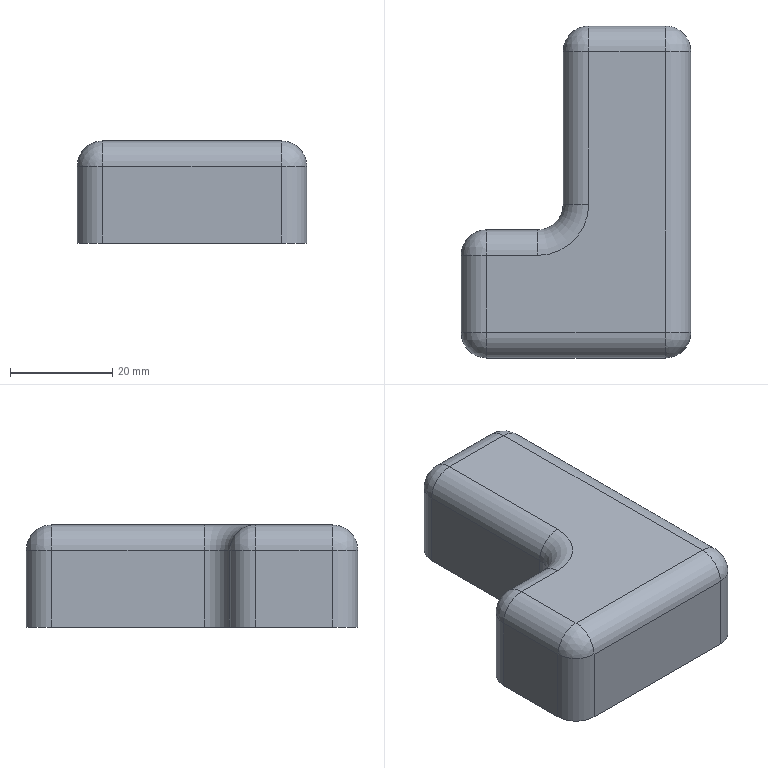Part | SolidWorks | features BaseBody 1 | 1 solid | 26 faces | box 45 x 65 x 20 mm | volume 41025 mm3 | cylinder 12 | plane 8 | sphere 5 | torus 1 | commonest cylinder face diameters 10 x12
STEP:
#1=CARTESIAN_POINT('',(40.,0.,15.));
#2=VERTEX_POINT('',#1);
#3=CARTESIAN_POINT('',(5.,0.,15.));
#4=VERTEX_POINT('',#3);
#5=CARTESIAN_POINT('',(45.,0.,15.));
#6=DIRECTION('',(-1.,0.,0.));
#7=VECTOR('',#6,1000.);
#8=LINE('',#5,#7);
#9=EDGE_CURVE('',#2,#4,#8,.T.);
#10=ORIENTED_EDGE('',*,*,#9,.T.);
#11=CARTESIAN_POINT('',(5.,0.,0.));
#12=VERTEX_POINT('',#11);
#13=CARTESIAN_POINT('',(5.,0.,20.));
#14=DIRECTION('',(0.,0.,-1.));
#15=VECTOR('',#14,1000.);
#16=LINE('',#13,#15);
#17=EDGE_CURVE('',#4,#12,#16,.T.);
#18=ORIENTED_EDGE('',*,*,#17,.T.);
#19=CARTESIAN_POINT('',(40.,0.,0.));
#20=VERTEX_POINT('',#19);
#21=CARTESIAN_POINT('',(45.,0.,0.));
#22=DIRECTION('',(1.,0.,0.));
#23=VECTOR('',#22,1000.);
#24=LINE('',#21,#23);
#25=EDGE_CURVE('',#12,#20,#24,.T.);
#26=ORIENTED_EDGE('',*,*,#25,.T.);
#27=CARTESIAN_POINT('',(40.,0.,20.));
#28=DIRECTION('',(0.,0.,1.));
#29=VECTOR('',#28,1000.);
#30=LINE('',#27,#29);
#31=EDGE_CURVE('',#20,#2,#30,.T.);
#32=ORIENTED_EDGE('',*,*,#31,.T.);
#33=EDGE_LOOP('',(#10,#18,#26,#32));
#34=FACE_OUTER_BOUND('',#33,.T.);
#35=CARTESIAN_POINT('',(45.,0.,20.));
#36=DIRECTION('',(0.,1.,0.));
#37=DIRECTION('',(-1.,0.,0.));
#38=AXIS2_PLACEMENT_3D('',#35,#36,#37);
#39=PLANE('',#38);
#40=ADVANCED_FACE('',(#34),#39,.F.);
#41=CARTESIAN_POINT('',(45.,60.,15.));
#42=VERTEX_POINT('',#41);
#43=CARTESIAN_POINT('',(45.,5.,15.));
#44=VERTEX_POINT('',#43);
#45=CARTESIAN_POINT('',(45.,65.,15.));
#46=DIRECTION('',(0.,-1.,0.));
#47=VECTOR('',#46,1000.);
#48=LINE('',#45,#47);
#49=EDGE_CURVE('',#42,#44,#48,.T.);
#50=ORIENTED_EDGE('',*,*,#49,.T.);
#51=CARTESIAN_POINT('',(45.,5.,0.));
#52=VERTEX_POINT('',#51);
#53=CARTESIAN_POINT('',(45.,5.,20.));
#54=DIRECTION('',(0.,0.,-1.));
#55=VECTOR('',#54,1000.);
#56=LINE('',#53,#55);
#57=EDGE_CURVE('',#44,#52,#56,.T.);
#58=ORIENTED_EDGE('',*,*,#57,.T.);
#59=CARTESIAN_POINT('',(45.,60.,0.));
#60=VERTEX_POINT('',#59);
#61=CARTESIAN_POINT('',(45.,65.,0.));
#62=DIRECTION('',(0.,1.,0.));
#63=VECTOR('',#62,1000.);
#64=LINE('',#61,#63);
#65=EDGE_CURVE('',#52,#60,#64,.T.);
#66=ORIENTED_EDGE('',*,*,#65,.T.);
#67=CARTESIAN_POINT('',(45.,60.,20.));
#68=DIRECTION('',(0.,0.,1.));
#69=VECTOR('',#68,1000.);
#70=LINE('',#67,#69);
#71=EDGE_CURVE('',#60,#42,#70,.T.);
#72=ORIENTED_EDGE('',*,*,#71,.T.);
#73=EDGE_LOOP('',(#50,#58,#66,#72));
#74=FACE_OUTER_BOUND('',#73,.T.);
#75=CARTESIAN_POINT('',(45.,65.,20.));
#76=DIRECTION('',(-1.,0.,0.));
#77=DIRECTION('',(0.,-1.,0.));
#78=AXIS2_PLACEMENT_3D('',#75,#76,#77);
#79=PLANE('',#78);
#80=ADVANCED_FACE('',(#74),#79,.F.);
#81=CARTESIAN_POINT('',(25.,65.,15.));
#82=VERTEX_POINT('',#81);
#83=CARTESIAN_POINT('',(40.,65.,15.));
#84=VERTEX_POINT('',#83);
#85=CARTESIAN_POINT('',(20.,65.,15.));
#86=DIRECTION('',(1.,0.,0.));
#87=VECTOR('',#86,1000.);
#88=LINE('',#85,#87);
#89=EDGE_CURVE('',#82,#84,#88,.T.);
#90=ORIENTED_EDGE('',*,*,#89,.T.);
#91=CARTESIAN_POINT('',(40.,65.,0.));
#92=VERTEX_POINT('',#91);
#93=CARTESIAN_POINT('',(40.,65.,20.));
#94=DIRECTION('',(0.,0.,-1.));
#95=VECTOR('',#94,1000.);
#96=LINE('',#93,#95);
#97=EDGE_CURVE('',#84,#92,#96,.T.);
#98=ORIENTED_EDGE('',*,*,#97,.T.);
#99=CARTESIAN_POINT('',(25.,65.,0.));
#100=VERTEX_POINT('',#99);
#101=CARTESIAN_POINT('',(20.,65.,0.));
#102=DIRECTION('',(-1.,0.,0.));
#103=VECTOR('',#102,1000.);
#104=LINE('',#101,#103);
#105=EDGE_CURVE('',#92,#100,#104,.T.);
#106=ORIENTED_EDGE('',*,*,#105,.T.);
#107=CARTESIAN_POINT('',(25.,65.,20.));
#108=DIRECTION('',(0.,0.,1.));
#109=VECTOR('',#108,1000.);
#110=LINE('',#107,#109);
#111=EDGE_CURVE('',#100,#82,#110,.T.);
#112=ORIENTED_EDGE('',*,*,#111,.T.);
#113=EDGE_LOOP('',(#90,#98,#106,#112));
#114=FACE_OUTER_BOUND('',#113,.T.);
#115=CARTESIAN_POINT('',(20.,65.,20.));
#116=DIRECTION('',(0.,-1.,0.));
#117=DIRECTION('',(0.,0.,-1.));
#118=AXIS2_PLACEMENT_3D('',#115,#116,#117);
#119=PLANE('',#118);
#120=ADVANCED_FACE('',(#114),#119,.F.);
#121=CARTESIAN_POINT('',(20.,30.07,15.));
#122=VERTEX_POINT('',#121);
#123=CARTESIAN_POINT('',(20.,60.,15.));
#124=VERTEX_POINT('',#123);
#125=CARTESIAN_POINT('',(20.,25.07,15.));
#126=DIRECTION('',(0.,1.,0.));
#127=VECTOR('',#126,1000.);
#128=LINE('',#125,#127);
#129=EDGE_CURVE('',#122,#124,#128,.T.);
#130=ORIENTED_EDGE('',*,*,#129,.T.);
#131=CARTESIAN_POINT('',(20.,60.,0.));
#132=VERTEX_POINT('',#131);
#133=CARTESIAN_POINT('',(20.,60.,20.));
#134=DIRECTION('',(0.,0.,-1.));
#135=VECTOR('',#134,1000.);
#136=LINE('',#133,#135);
#137=EDGE_CURVE('',#124,#132,#136,.T.);
#138=ORIENTED_EDGE('',*,*,#137,.T.);
#139=CARTESIAN_POINT('',(20.,30.07,0.));
#140=VERTEX_POINT('',#139);
#141=CARTESIAN_POINT('',(20.,25.07,0.));
#142=DIRECTION('',(0.,-1.,0.));
#143=VECTOR('',#142,1000.);
#144=LINE('',#141,#143);
#145=EDGE_CURVE('',#132,#140,#144,.T.);
#146=ORIENTED_EDGE('',*,*,#145,.T.);
#147=CARTESIAN_POINT('',(20.,30.07,20.));
#148=DIRECTION('',(0.,0.,1.));
#149=VECTOR('',#148,1000.);
#150=LINE('',#147,#149);
#151=EDGE_CURVE('',#140,#122,#150,.T.);
#152=ORIENTED_EDGE('',*,*,#151,.T.);
#153=EDGE_LOOP('',(#130,#138,#146,#152));
#154=FACE_OUTER_BOUND('',#153,.T.);
#155=CARTESIAN_POINT('',(20.,25.07,20.));
#156=DIRECTION('',(1.,0.,0.));
#157=DIRECTION('',(0.,0.,-1.));
#158=AXIS2_PLACEMENT_3D('',#155,#156,#157);
#159=PLANE('',#158);
#160=ADVANCED_FACE('',(#154),#159,.F.);
#161=CARTESIAN_POINT('',(5.,25.07,15.));
#162=VERTEX_POINT('',#161);
#163=CARTESIAN_POINT('',(15.,25.07,15.));
#164=VERTEX_POINT('',#163);
#165=CARTESIAN_POINT('',(0.,25.07,15.));
#166=DIRECTION('',(1.,0.,0.));
#167=VECTOR('',#166,1000.);
#168=LINE('',#165,#167);
#169=EDGE_CURVE('',#162,#164,#168,.T.);
#170=ORIENTED_EDGE('',*,*,#169,.T.);
#171=CARTESIAN_POINT('',(15.,25.07,0.));
#172=VERTEX_POINT('',#171);
#173=CARTESIAN_POINT('',(15.,25.07,0.));
#174=DIRECTION('',(0.,0.,-1.));
#175=VECTOR('',#174,1000.);
#176=LINE('',#173,#175);
#177=EDGE_CURVE('',#164,#172,#176,.T.);
#178=ORIENTED_EDGE('',*,*,#177,.T.);
#179=CARTESIAN_POINT('',(5.,25.07,0.));
#180=VERTEX_POINT('',#179);
#181=CARTESIAN_POINT('',(0.,25.07,0.));
#182=DIRECTION('',(-1.,0.,0.));
#183=VECTOR('',#182,1000.);
#184=LINE('',#181,#183);
#185=EDGE_CURVE('',#172,#180,#184,.T.);
#186=ORIENTED_EDGE('',*,*,#185,.T.);
#187=CARTESIAN_POINT('',(5.,25.07,20.));
#188=DIRECTION('',(0.,0.,1.));
#189=VECTOR('',#188,1000.);
#190=LINE('',#187,#189);
#191=EDGE_CURVE('',#180,#162,#190,.T.);
#192=ORIENTED_EDGE('',*,*,#191,.T.);
#193=EDGE_LOOP('',(#170,#178,#186,#192));
#194=FACE_OUTER_BOUND('',#193,.T.);
#195=CARTESIAN_POINT('',(0.,25.07,20.));
#196=DIRECTION('',(0.,-1.,0.));
#197=DIRECTION('',(0.,0.,-1.));
#198=AXIS2_PLACEMENT_3D('',#195,#196,#197);
#199=PLANE('',#198);
#200=ADVANCED_FACE('',(#194),#199,.F.);
#201=CARTESIAN_POINT('',(0.,20.07,0.));
#202=VERTEX_POINT('',#201);
#203=CARTESIAN_POINT('',(0.,5.,0.));
#204=VERTEX_POINT('',#203);
#205=CARTESIAN_POINT('',(0.,0.,0.));
#206=DIRECTION('',(0.,-1.,0.));
#207=VECTOR('',#206,1000.);
#208=LINE('',#205,#207);
#209=EDGE_CURVE('',#202,#204,#208,.T.);
#210=ORIENTED_EDGE('',*,*,#209,.T.);
#211=CARTESIAN_POINT('',(0.,5.,15.));
#212=VERTEX_POINT('',#211);
#213=CARTESIAN_POINT('',(0.,5.,20.));
#214=DIRECTION('',(0.,0.,1.));
#215=VECTOR('',#214,1000.);
#216=LINE('',#213,#215);
#217=EDGE_CURVE('',#204,#212,#216,.T.);
#218=ORIENTED_EDGE('',*,*,#217,.T.);
#219=CARTESIAN_POINT('',(0.,20.07,15.));
#220=VERTEX_POINT('',#219);
#221=CARTESIAN_POINT('',(0.,0.,15.));
#222=DIRECTION('',(0.,1.,0.));
#223=VECTOR('',#222,1000.);
#224=LINE('',#221,#223);
#225=EDGE_CURVE('',#212,#220,#224,.T.);
#226=ORIENTED_EDGE('',*,*,#225,.T.);
#227=CARTESIAN_POINT('',(0.,20.07,20.));
#228=DIRECTION('',(0.,0.,-1.));
#229=VECTOR('',#228,1000.);
#230=LINE('',#227,#229);
#231=EDGE_CURVE('',#220,#202,#230,.T.);
#232=ORIENTED_EDGE('',*,*,#231,.T.);
#233=EDGE_LOOP('',(#210,#218,#226,#232));
#234=FACE_OUTER_BOUND('',#233,.T.);
#235=CARTESIAN_POINT('',(0.,0.,20.));
#236=DIRECTION('',(1.,0.,0.));
#237=DIRECTION('',(0.,0.,-1.));
#238=AXIS2_PLACEMENT_3D('',#235,#236,#237);
#239=PLANE('',#238);
#240=ADVANCED_FACE('',(#234),#239,.F.);
#241=CARTESIAN_POINT('',(40.,60.,20.));
#242=VERTEX_POINT('',#241);
#243=CARTESIAN_POINT('',(25.,60.,20.));
#244=VERTEX_POINT('',#243);
#245=CARTESIAN_POINT('',(0.,60.,20.));
#246=DIRECTION('',(-1.,0.,0.));
#247=VECTOR('',#246,1000.);
#248=LINE('',#245,#247);
#249=EDGE_CURVE('',#242,#244,#248,.T.);
#250=ORIENTED_EDGE('',*,*,#249,.T.);
#251=CARTESIAN_POINT('',(25.,30.07,20.));
#252=VERTEX_POINT('',#251);
#253=CARTESIAN_POINT('',(25.,0.,20.));
#254=DIRECTION('',(0.,-1.,0.));
#255=VECTOR('',#254,1000.);
#256=LINE('',#253,#255);
#257=EDGE_CURVE('',#244,#252,#256,.T.);
#258=ORIENTED_EDGE('',*,*,#257,.T.);
#259=CARTESIAN_POINT('',(15.,20.07,20.));
#260=VERTEX_POINT('',#259);
#261=CARTESIAN_POINT('',(15.,30.07,20.));
#262=DIRECTION('',(0.,0.,1.));
#263=DIRECTION('',(-1.,0.,0.));
#264=AXIS2_PLACEMENT_3D('',#261,#262,#263);
#265=CIRCLE('',#264,10.);
#266=EDGE_CURVE('',#260,#252,#265,.T.);
#267=ORIENTED_EDGE('',*,*,#266,.F.);
#268=CARTESIAN_POINT('',(5.,20.07,20.));
#269=VERTEX_POINT('',#268);
#270=CARTESIAN_POINT('',(0.,20.07,20.));
#271=DIRECTION('',(-1.,0.,0.));
#272=VECTOR('',#271,1000.);
#273=LINE('',#270,#272);
#274=EDGE_CURVE('',#260,#269,#273,.T.);
#275=ORIENTED_EDGE('',*,*,#274,.T.);
#276=CARTESIAN_POINT('',(5.,5.,20.));
#277=VERTEX_POINT('',#276);
#278=CARTESIAN_POINT('',(5.,0.,20.));
#279=DIRECTION('',(0.,-1.,0.));
#280=VECTOR('',#279,1000.);
#281=LINE('',#278,#280);
#282=EDGE_CURVE('',#269,#277,#281,.T.);
#283=ORIENTED_EDGE('',*,*,#282,.T.);
#284=CARTESIAN_POINT('',(40.,5.,20.));
#285=VERTEX_POINT('',#284);
#286=CARTESIAN_POINT('',(0.,5.,20.));
#287=DIRECTION('',(1.,0.,0.));
#288=VECTOR('',#287,1000.);
#289=LINE('',#286,#288);
#290=EDGE_CURVE('',#277,#285,#289,.T.);
#291=ORIENTED_EDGE('',*,*,#290,.T.);
#292=CARTESIAN_POINT('',(40.,0.,20.));
#293=DIRECTION('',(0.,1.,0.));
#294=VECTOR('',#293,1000.);
#295=LINE('',#292,#294);
#296=EDGE_CURVE('',#285,#242,#295,.T.);
#297=ORIENTED_EDGE('',*,*,#296,.T.);
#298=EDGE_LOOP('',(#250,#258,#267,#275,#283,#291,#297));
#299=FACE_OUTER_BOUND('',#298,.T.);
#300=CARTESIAN_POINT('',(0.,0.,20.));
#301=DIRECTION('',(0.,0.,-1.));
#302=DIRECTION('',(-1.,0.,0.));
#303=AXIS2_PLACEMENT_3D('',#300,#301,#302);
#304=PLANE('',#303);
#305=ADVANCED_FACE('',(#299),#304,.F.);
#306=ORIENTED_EDGE('',*,*,#25,.F.);
#307=CARTESIAN_POINT('',(5.,5.,0.));
#308=DIRECTION('',(0.,0.,-1.));
#309=DIRECTION('',(-1.,0.,0.));
#310=AXIS2_PLACEMENT_3D('',#307,#308,#309);
#311=CIRCLE('',#310,5.);
#312=EDGE_CURVE('',#12,#204,#311,.T.);
#313=ORIENTED_EDGE('',*,*,#312,.T.);
#314=ORIENTED_EDGE('',*,*,#209,.F.);
#315=CARTESIAN_POINT('',(5.,20.07,0.));
#316=DIRECTION('',(0.,0.,-1.));
#317=DIRECTION('',(-1.,0.,0.));
#318=AXIS2_PLACEMENT_3D('',#315,#316,#317);
#319=CIRCLE('',#318,5.);
#320=EDGE_CURVE('',#202,#180,#319,.T.);
#321=ORIENTED_EDGE('',*,*,#320,.T.);
#322=ORIENTED_EDGE('',*,*,#185,.F.);
#323=CARTESIAN_POINT('',(15.,30.07,0.));
#324=DIRECTION('',(0.,0.,1.));
#325=DIRECTION('',(-1.,0.,0.));
#326=AXIS2_PLACEMENT_3D('',#323,#324,#325);
#327=CIRCLE('',#326,5.);
#328=EDGE_CURVE('',#172,#140,#327,.T.);
#329=ORIENTED_EDGE('',*,*,#328,.T.);
#330=ORIENTED_EDGE('',*,*,#145,.F.);
#331=CARTESIAN_POINT('',(25.,60.,0.));
#332=DIRECTION('',(0.,0.,-1.));
#333=DIRECTION('',(-1.,0.,0.));
#334=AXIS2_PLACEMENT_3D('',#331,#332,#333);
#335=CIRCLE('',#334,5.);
#336=EDGE_CURVE('',#132,#100,#335,.T.);
#337=ORIENTED_EDGE('',*,*,#336,.T.);
#338=ORIENTED_EDGE('',*,*,#105,.F.);
#339=CARTESIAN_POINT('',(40.,60.,0.));
#340=DIRECTION('',(0.,0.,-1.));
#341=DIRECTION('',(-1.,0.,0.));
#342=AXIS2_PLACEMENT_3D('',#339,#340,#341);
#343=CIRCLE('',#342,5.);
#344=EDGE_CURVE('',#92,#60,#343,.T.);
#345=ORIENTED_EDGE('',*,*,#344,.T.);
#346=ORIENTED_EDGE('',*,*,#65,.F.);
#347=CARTESIAN_POINT('',(40.,5.,0.));
#348=DIRECTION('',(0.,0.,-1.));
#349=DIRECTION('',(-1.,0.,0.));
#350=AXIS2_PLACEMENT_3D('',#347,#348,#349);
#351=CIRCLE('',#350,5.);
#352=EDGE_CURVE('',#52,#20,#351,.T.);
#353=ORIENTED_EDGE('',*,*,#352,.T.);
#354=EDGE_LOOP('',(#306,#313,#314,#321,#322,#329,#330,#337,#338,#345,#346,#353));
#355=FACE_OUTER_BOUND('',#354,.T.);
#356=CARTESIAN_POINT('',(0.,0.,0.));
#357=DIRECTION('',(0.,0.,-1.));
#358=DIRECTION('',(-1.,0.,0.));
#359=AXIS2_PLACEMENT_3D('',#356,#357,#358);
#360=PLANE('',#359);
#361=ADVANCED_FACE('',(#355),#360,.T.);
#362=ORIENTED_EDGE('',*,*,#352,.F.);
#363=ORIENTED_EDGE('',*,*,#57,.F.);
#364=CARTESIAN_POINT('',(40.,5.,15.));
#365=DIRECTION('',(0.,0.,1.));
#366=DIRECTION('',(1.,0.,0.));
#367=AXIS2_PLACEMENT_3D('',#364,#365,#366);
#368=CIRCLE('',#367,5.);
#369=EDGE_CURVE('',#2,#44,#368,.T.);
#370=ORIENTED_EDGE('',*,*,#369,.F.);
#371=ORIENTED_EDGE('',*,*,#31,.F.);
#372=EDGE_LOOP('',(#362,#363,#370,#371));
#373=FACE_OUTER_BOUND('',#372,.T.);
#374=CARTESIAN_POINT('',(40.,5.,20.));
#375=DIRECTION('',(0.,0.,-1.));
#376=DIRECTION('',(-1.,0.,0.));
#377=AXIS2_PLACEMENT_3D('',#374,#375,#376);
#378=CYLINDRICAL_SURFACE('',#377,5.);
#379=ADVANCED_FACE('',(#373),#378,.T.);
#380=CARTESIAN_POINT('',(5.,5.,15.));
#381=DIRECTION('',(-1.,0.,0.));
#382=DIRECTION('',(0.,0.,1.));
#383=AXIS2_PLACEMENT_3D('',#380,#381,#382);
#384=CIRCLE('',#383,5.);
#385=EDGE_CURVE('',#4,#277,#384,.T.);
#386=ORIENTED_EDGE('',*,*,#385,.F.);
#387=ORIENTED_EDGE('',*,*,#9,.F.);
#388=CARTESIAN_POINT('',(40.,5.,15.));
#389=DIRECTION('',(1.,0.,0.));
#390=DIRECTION('',(0.,0.,-1.));
#391=AXIS2_PLACEMENT_3D('',#388,#389,#390);
#392=CIRCLE('',#391,5.);
#393=EDGE_CURVE('',#285,#2,#392,.T.);
#394=ORIENTED_EDGE('',*,*,#393,.F.);
#395=ORIENTED_EDGE('',*,*,#290,.F.);
#396=EDGE_LOOP('',(#386,#387,#394,#395));
#397=FACE_OUTER_BOUND('',#396,.T.);
#398=CARTESIAN_POINT('',(0.,5.,15.));
#399=DIRECTION('',(1.,0.,0.));
#400=DIRECTION('',(0.,1.,0.));
#401=AXIS2_PLACEMENT_3D('',#398,#399,#400);
#402=CYLINDRICAL_SURFACE('',#401,5.);
#403=ADVANCED_FACE('',(#397),#402,.T.);
#404=ORIENTED_EDGE('',*,*,#312,.F.);
#405=ORIENTED_EDGE('',*,*,#17,.F.);
#406=CARTESIAN_POINT('',(5.,5.,15.));
#407=DIRECTION('',(0.,0.,1.));
#408=DIRECTION('',(1.,0.,0.));
#409=AXIS2_PLACEMENT_3D('',#406,#407,#408);
#410=CIRCLE('',#409,5.);
#411=EDGE_CURVE('',#212,#4,#410,.T.);
#412=ORIENTED_EDGE('',*,*,#411,.F.);
#413=ORIENTED_EDGE('',*,*,#217,.F.);
#414=EDGE_LOOP('',(#404,#405,#412,#413));
#415=FACE_OUTER_BOUND('',#414,.T.);
#416=CARTESIAN_POINT('',(5.,5.,20.));
#417=DIRECTION('',(0.,0.,-1.));
#418=DIRECTION('',(-1.,0.,0.));
#419=AXIS2_PLACEMENT_3D('',#416,#417,#418);
#420=CYLINDRICAL_SURFACE('',#419,5.);
#421=ADVANCED_FACE('',(#415),#420,.T.);
#422=ORIENTED_EDGE('',*,*,#393,.T.);
#423=ORIENTED_EDGE('',*,*,#369,.T.);
#424=CARTESIAN_POINT('',(40.,5.,15.));
#425=DIRECTION('',(0.,1.,0.));
#426=DIRECTION('',(0.,0.,-1.));
#427=AXIS2_PLACEMENT_3D('',#424,#425,#426);
#428=CIRCLE('',#427,5.);
#429=EDGE_CURVE('',#285,#44,#428,.T.);
#430=ORIENTED_EDGE('',*,*,#429,.F.);
#431=EDGE_LOOP('',(#422,#423,#430));
#432=FACE_OUTER_BOUND('',#431,.T.);
#433=CARTESIAN_POINT('',(40.,5.,15.));
#434=DIRECTION('',(0.,1.,0.));
#435=DIRECTION('',(1.,0.,0.));
#436=AXIS2_PLACEMENT_3D('',#433,#434,#435);
#437=SPHERICAL_SURFACE('',#436,5.);
#438=ADVANCED_FACE('',(#432),#437,.T.);
#439=ORIENTED_EDGE('',*,*,#411,.T.);
#440=ORIENTED_EDGE('',*,*,#385,.T.);
#441=CARTESIAN_POINT('',(5.,5.,15.));
#442=DIRECTION('',(0.,1.,0.));
#443=DIRECTION('',(0.,0.,-1.));
#444=AXIS2_PLACEMENT_3D('',#441,#442,#443);
#445=CIRCLE('',#444,5.);
#446=EDGE_CURVE('',#212,#277,#445,.T.);
#447=ORIENTED_EDGE('',*,*,#446,.F.);
#448=EDGE_LOOP('',(#439,#440,#447));
#449=FACE_OUTER_BOUND('',#448,.T.);
#450=CARTESIAN_POINT('',(5.,5.,15.));
#451=DIRECTION('',(0.,1.,0.));
#452=DIRECTION('',(1.,0.,0.));
#453=AXIS2_PLACEMENT_3D('',#450,#451,#452);
#454=SPHERICAL_SURFACE('',#453,5.);
#455=ADVANCED_FACE('',(#449),#454,.T.);
#456=ORIENTED_EDGE('',*,*,#344,.F.);
#457=ORIENTED_EDGE('',*,*,#97,.F.);
#458=CARTESIAN_POINT('',(40.,60.,15.));
#459=DIRECTION('',(0.,0.,1.));
#460=DIRECTION('',(1.,0.,0.));
#461=AXIS2_PLACEMENT_3D('',#458,#459,#460);
#462=CIRCLE('',#461,5.);
#463=EDGE_CURVE('',#42,#84,#462,.T.);
#464=ORIENTED_EDGE('',*,*,#463,.F.);
#465=ORIENTED_EDGE('',*,*,#71,.F.);
#466=EDGE_LOOP('',(#456,#457,#464,#465));
#467=FACE_OUTER_BOUND('',#466,.T.);
#468=CARTESIAN_POINT('',(40.,60.,20.));
#469=DIRECTION('',(0.,0.,-1.));
#470=DIRECTION('',(-1.,0.,0.));
#471=AXIS2_PLACEMENT_3D('',#468,#469,#470);
#472=CYLINDRICAL_SURFACE('',#471,5.);
#473=ADVANCED_FACE('',(#467),#472,.T.);
#474=ORIENTED_EDGE('',*,*,#429,.T.);
#475=ORIENTED_EDGE('',*,*,#49,.F.);
#476=CARTESIAN_POINT('',(40.,60.,15.));
#477=DIRECTION('',(0.,1.,0.));
#478=DIRECTION('',(0.,0.,1.));
#479=AXIS2_PLACEMENT_3D('',#476,#477,#478);
#480=CIRCLE('',#479,5.);
#481=EDGE_CURVE('',#242,#42,#480,.T.);
#482=ORIENTED_EDGE('',*,*,#481,.F.);
#483=ORIENTED_EDGE('',*,*,#296,.F.);
#484=EDGE_LOOP('',(#474,#475,#482,#483));
#485=FACE_OUTER_BOUND('',#484,.T.);
#486=CARTESIAN_POINT('',(40.,0.,15.));
#487=DIRECTION('',(0.,1.,0.));
#488=DIRECTION('',(-1.,0.,0.));
#489=AXIS2_PLACEMENT_3D('',#486,#487,#488);
#490=CYLINDRICAL_SURFACE('',#489,5.);
#491=ADVANCED_FACE('',(#485),#490,.T.);
#492=ORIENTED_EDGE('',*,*,#446,.T.);
#493=ORIENTED_EDGE('',*,*,#282,.F.);
#494=CARTESIAN_POINT('',(5.,20.07,15.));
#495=DIRECTION('',(0.,1.,0.));
#496=DIRECTION('',(0.,0.,1.));
#497=AXIS2_PLACEMENT_3D('',#494,#495,#496);
#498=CIRCLE('',#497,5.);
#499=EDGE_CURVE('',#220,#269,#498,.T.);
#500=ORIENTED_EDGE('',*,*,#499,.F.);
#501=ORIENTED_EDGE('',*,*,#225,.F.);
#502=EDGE_LOOP('',(#492,#493,#500,#501));
#503=FACE_OUTER_BOUND('',#502,.T.);
#504=CARTESIAN_POINT('',(5.,0.,15.));
#505=DIRECTION('',(0.,-1.,0.));
#506=DIRECTION('',(0.,0.,-1.));
#507=AXIS2_PLACEMENT_3D('',#504,#505,#506);
#508=CYLINDRICAL_SURFACE('',#507,5.);
#509=ADVANCED_FACE('',(#503),#508,.T.);
#510=ORIENTED_EDGE('',*,*,#320,.F.);
#511=ORIENTED_EDGE('',*,*,#231,.F.);
#512=CARTESIAN_POINT('',(5.,20.07,15.));
#513=DIRECTION('',(0.,0.,1.));
#514=DIRECTION('',(1.,0.,0.));
#515=AXIS2_PLACEMENT_3D('',#512,#513,#514);
#516=CIRCLE('',#515,5.);
#517=EDGE_CURVE('',#162,#220,#516,.T.);
#518=ORIENTED_EDGE('',*,*,#517,.F.);
#519=ORIENTED_EDGE('',*,*,#191,.F.);
#520=EDGE_LOOP('',(#510,#511,#518,#519));
#521=FACE_OUTER_BOUND('',#520,.T.);
#522=CARTESIAN_POINT('',(5.,20.07,20.));
#523=DIRECTION('',(0.,0.,-1.));
#524=DIRECTION('',(-1.,0.,0.));
#525=AXIS2_PLACEMENT_3D('',#522,#523,#524);
#526=CYLINDRICAL_SURFACE('',#525,5.);
#527=ADVANCED_FACE('',(#521),#526,.T.);
#528=ORIENTED_EDGE('',*,*,#481,.T.);
#529=ORIENTED_EDGE('',*,*,#463,.T.);
#530=CARTESIAN_POINT('',(40.,60.,15.));
#531=DIRECTION('',(-1.,0.,0.));
#532=DIRECTION('',(0.,0.,-1.));
#533=AXIS2_PLACEMENT_3D('',#530,#531,#532);
#534=CIRCLE('',#533,5.);
#535=EDGE_CURVE('',#242,#84,#534,.T.);
#536=ORIENTED_EDGE('',*,*,#535,.F.);
#537=EDGE_LOOP('',(#528,#529,#536));
#538=FACE_OUTER_BOUND('',#537,.T.);
#539=CARTESIAN_POINT('',(40.,60.,15.));
#540=DIRECTION('',(0.,1.,0.));
#541=DIRECTION('',(1.,0.,0.));
#542=AXIS2_PLACEMENT_3D('',#539,#540,#541);
#543=SPHERICAL_SURFACE('',#542,5.);
#544=ADVANCED_FACE('',(#538),#543,.T.);
#545=ORIENTED_EDGE('',*,*,#517,.T.);
#546=ORIENTED_EDGE('',*,*,#499,.T.);
#547=CARTESIAN_POINT('',(5.,20.07,15.));
#548=DIRECTION('',(1.,0.,0.));
#549=DIRECTION('',(0.,0.,1.));
#550=AXIS2_PLACEMENT_3D('',#547,#548,#549);
#551=CIRCLE('',#550,5.);
#552=EDGE_CURVE('',#162,#269,#551,.T.);
#553=ORIENTED_EDGE('',*,*,#552,.F.);
#554=EDGE_LOOP('',(#545,#546,#553));
#555=FACE_OUTER_BOUND('',#554,.T.);
#556=CARTESIAN_POINT('',(5.,20.07,15.));
#557=DIRECTION('',(0.,1.,0.));
#558=DIRECTION('',(1.,0.,0.));
#559=AXIS2_PLACEMENT_3D('',#556,#557,#558);
#560=SPHERICAL_SURFACE('',#559,5.);
#561=ADVANCED_FACE('',(#555),#560,.T.);
#562=ORIENTED_EDGE('',*,*,#336,.F.);
#563=ORIENTED_EDGE('',*,*,#137,.F.);
#564=CARTESIAN_POINT('',(25.,60.,15.));
#565=DIRECTION('',(0.,0.,1.));
#566=DIRECTION('',(1.,0.,0.));
#567=AXIS2_PLACEMENT_3D('',#564,#565,#566);
#568=CIRCLE('',#567,5.);
#569=EDGE_CURVE('',#82,#124,#568,.T.);
#570=ORIENTED_EDGE('',*,*,#569,.F.);
#571=ORIENTED_EDGE('',*,*,#111,.F.);
#572=EDGE_LOOP('',(#562,#563,#570,#571));
#573=FACE_OUTER_BOUND('',#572,.T.);
#574=CARTESIAN_POINT('',(25.,60.,20.));
#575=DIRECTION('',(0.,0.,-1.));
#576=DIRECTION('',(-1.,0.,0.));
#577=AXIS2_PLACEMENT_3D('',#574,#575,#576);
#578=CYLINDRICAL_SURFACE('',#577,5.);
#579=ADVANCED_FACE('',(#573),#578,.T.);
#580=ORIENTED_EDGE('',*,*,#535,.T.);
#581=ORIENTED_EDGE('',*,*,#89,.F.);
#582=CARTESIAN_POINT('',(25.,60.,15.));
#583=DIRECTION('',(-1.,0.,0.));
#584=DIRECTION('',(0.,0.,1.));
#585=AXIS2_PLACEMENT_3D('',#582,#583,#584);
#586=CIRCLE('',#585,5.);
#587=EDGE_CURVE('',#244,#82,#586,.T.);
#588=ORIENTED_EDGE('',*,*,#587,.F.);
#589=ORIENTED_EDGE('',*,*,#249,.F.);
#590=EDGE_LOOP('',(#580,#581,#588,#589));
#591=FACE_OUTER_BOUND('',#590,.T.);
#592=CARTESIAN_POINT('',(0.,60.,15.));
#593=DIRECTION('',(-1.,0.,0.));
#594=DIRECTION('',(0.,0.,1.));
#595=AXIS2_PLACEMENT_3D('',#592,#593,#594);
#596=CYLINDRICAL_SURFACE('',#595,5.);
#597=ADVANCED_FACE('',(#591),#596,.T.);
#598=ORIENTED_EDGE('',*,*,#552,.T.);
#599=ORIENTED_EDGE('',*,*,#274,.F.);
#600=CARTESIAN_POINT('',(15.,20.07,15.));
#601=DIRECTION('',(1.,0.,0.));
#602=DIRECTION('',(0.,0.,-1.));
#603=AXIS2_PLACEMENT_3D('',#600,#601,#602);
#604=CIRCLE('',#603,5.);
#605=EDGE_CURVE('',#164,#260,#604,.T.);
#606=ORIENTED_EDGE('',*,*,#605,.F.);
#607=ORIENTED_EDGE('',*,*,#169,.F.);
#608=EDGE_LOOP('',(#598,#599,#606,#607));
#609=FACE_OUTER_BOUND('',#608,.T.);
#610=CARTESIAN_POINT('',(0.,20.07,15.));
#611=DIRECTION('',(-1.,0.,0.));
#612=DIRECTION('',(0.,0.,1.));
#613=AXIS2_PLACEMENT_3D('',#610,#611,#612);
#614=CYLINDRICAL_SURFACE('',#613,5.);
#615=ADVANCED_FACE('',(#609),#614,.T.);
#616=ORIENTED_EDGE('',*,*,#328,.F.);
#617=ORIENTED_EDGE('',*,*,#177,.F.);
#618=CARTESIAN_POINT('',(15.,30.07,15.));
#619=DIRECTION('',(0.,0.,-1.));
#620=DIRECTION('',(-1.,0.,0.));
#621=AXIS2_PLACEMENT_3D('',#618,#619,#620);
#622=CIRCLE('',#621,5.);
#623=EDGE_CURVE('',#122,#164,#622,.T.);
#624=ORIENTED_EDGE('',*,*,#623,.F.);
#625=ORIENTED_EDGE('',*,*,#151,.F.);
#626=EDGE_LOOP('',(#616,#617,#624,#625));
#627=FACE_OUTER_BOUND('',#626,.T.);
#628=CARTESIAN_POINT('',(15.,30.07,20.));
#629=DIRECTION('',(0.,0.,1.));
#630=DIRECTION('',(1.,0.,0.));
#631=AXIS2_PLACEMENT_3D('',#628,#629,#630);
#632=CYLINDRICAL_SURFACE('',#631,5.);
#633=ADVANCED_FACE('',(#627),#632,.F.);
#634=ORIENTED_EDGE('',*,*,#587,.T.);
#635=ORIENTED_EDGE('',*,*,#569,.T.);
#636=CARTESIAN_POINT('',(25.,60.,15.));
#637=DIRECTION('',(0.,-1.,0.));
#638=DIRECTION('',(0.,0.,1.));
#639=AXIS2_PLACEMENT_3D('',#636,#637,#638);
#640=CIRCLE('',#639,5.);
#641=EDGE_CURVE('',#244,#124,#640,.T.);
#642=ORIENTED_EDGE('',*,*,#641,.F.);
#643=EDGE_LOOP('',(#634,#635,#642));
#644=FACE_OUTER_BOUND('',#643,.T.);
#645=CARTESIAN_POINT('',(25.,60.,15.));
#646=DIRECTION('',(0.,1.,0.));
#647=DIRECTION('',(1.,0.,0.));
#648=AXIS2_PLACEMENT_3D('',#645,#646,#647);
#649=SPHERICAL_SURFACE('',#648,5.);
#650=ADVANCED_FACE('',(#644),#649,.T.);
#651=ORIENTED_EDGE('',*,*,#605,.T.);
#652=ORIENTED_EDGE('',*,*,#266,.T.);
#653=CARTESIAN_POINT('',(25.,30.07,15.));
#654=DIRECTION('',(0.,1.,0.));
#655=DIRECTION('',(0.,0.,-1.));
#656=AXIS2_PLACEMENT_3D('',#653,#654,#655);
#657=CIRCLE('',#656,5.);
#658=EDGE_CURVE('',#122,#252,#657,.T.);
#659=ORIENTED_EDGE('',*,*,#658,.F.);
#660=ORIENTED_EDGE('',*,*,#623,.T.);
#661=EDGE_LOOP('',(#651,#652,#659,#660));
#662=FACE_OUTER_BOUND('',#661,.T.);
#663=CARTESIAN_POINT('',(15.,30.07,15.));
#664=DIRECTION('',(0.,0.,-1.));
#665=DIRECTION('',(-1.,0.,0.));
#666=AXIS2_PLACEMENT_3D('',#663,#664,#665);
#667=TOROIDAL_SURFACE('',#666,10.,5.);
#668=ADVANCED_FACE('',(#662),#667,.T.);
#669=ORIENTED_EDGE('',*,*,#641,.T.);
#670=ORIENTED_EDGE('',*,*,#129,.F.);
#671=ORIENTED_EDGE('',*,*,#658,.T.);
#672=ORIENTED_EDGE('',*,*,#257,.F.);
#673=EDGE_LOOP('',(#669,#670,#671,#672));
#674=FACE_OUTER_BOUND('',#673,.T.);
#675=CARTESIAN_POINT('',(25.,0.,15.));
#676=DIRECTION('',(0.,-1.,0.));
#677=DIRECTION('',(0.,0.,-1.));
#678=AXIS2_PLACEMENT_3D('',#675,#676,#677);
#679=CYLINDRICAL_SURFACE('',#678,5.);
#680=ADVANCED_FACE('',(#674),#679,.T.);
#681=CLOSED_SHELL('',(#40,#80,#120,#160,#200,#240,#305,#361,#379,#403,#421,#438,#455,#473,#491,#509,#527,#544,#561,#579,#597,#615,#633,#650,#668,#680));
#682=MANIFOLD_SOLID_BREP('',#681);
#683=CARTESIAN_POINT('',(0.,0.,0.));
#684=DIRECTION('',(0.,0.,1.));
#685=DIRECTION('',(1.,0.,0.));
#686=AXIS2_PLACEMENT_3D('',#683,#684,#685);
#687=(LENGTH_UNIT()NAMED_UNIT(*)SI_UNIT(.MILLI.,.METRE.));
#688=UNCERTAINTY_MEASURE_WITH_UNIT(LENGTH_MEASURE(0.00001),#687,'','');
#689=(NAMED_UNIT(*)PLANE_ANGLE_UNIT()SI_UNIT($,.RADIAN.));
#690=(NAMED_UNIT(*)SI_UNIT($,.STERADIAN.)SOLID_ANGLE_UNIT());
#691=(GEOMETRIC_REPRESENTATION_CONTEXT(3)GLOBAL_UNCERTAINTY_ASSIGNED_CONTEXT((#688))GLOBAL_UNIT_ASSIGNED_CONTEXT((#687,#689,#690))REPRESENTATION_CONTEXT('',''));
#692=ADVANCED_BREP_SHAPE_REPRESENTATION('',(#682,#686),#691);